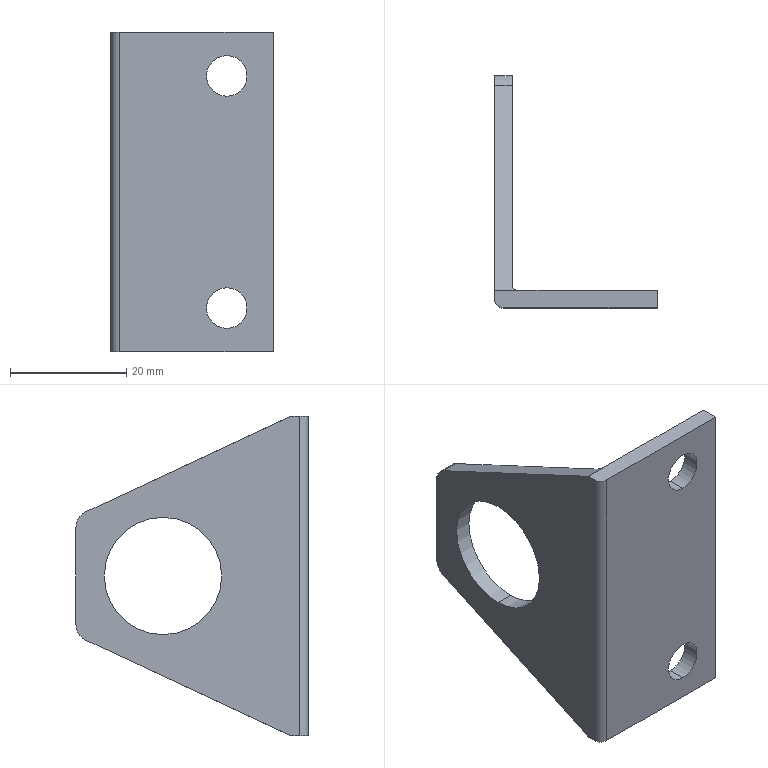Part | STEP file | F_MF20LB_RMS_ | 1 solid | 20 faces | box 28 x 40 x 55 mm | volume 7599 mm3 | cylinder 10 | plane 10 | commonest cylinder face diameters 7 x4 6 x2 20.2 x2 2 x1 3 x1